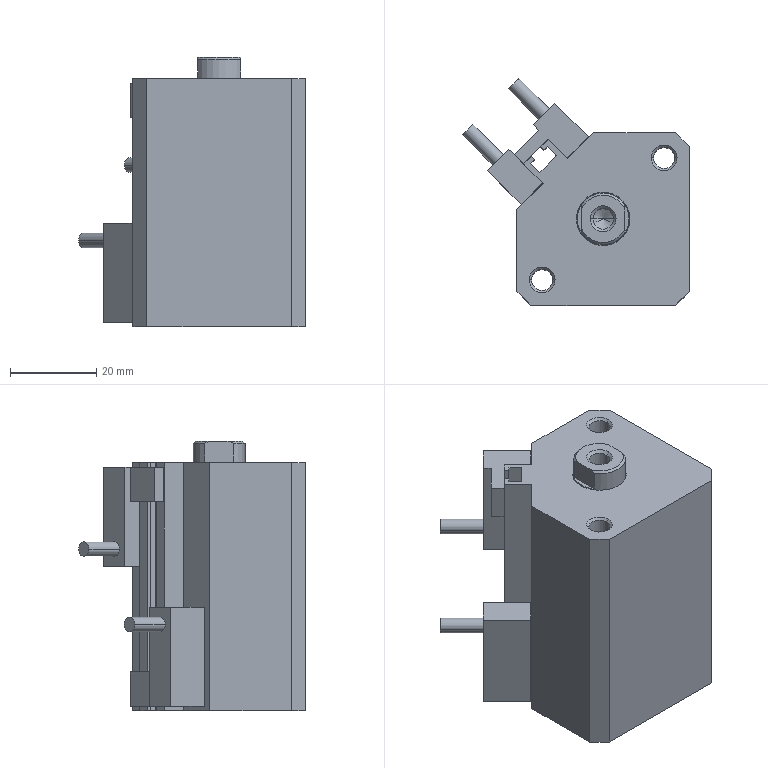Part | STEP file | A_CDQ2A25-25D-F7NV012_Default | 2 solids | 89 faces | box 52.598 x 52.598 x 62.5 mm | volume 85379 mm3 | plane 50 | cylinder 18 | cone 18 | spline 3 | commonest cylinder face diameters 3.4 x4 4.13 x4 4.92 x4 4.77 x2 12 x2 12.4 x2